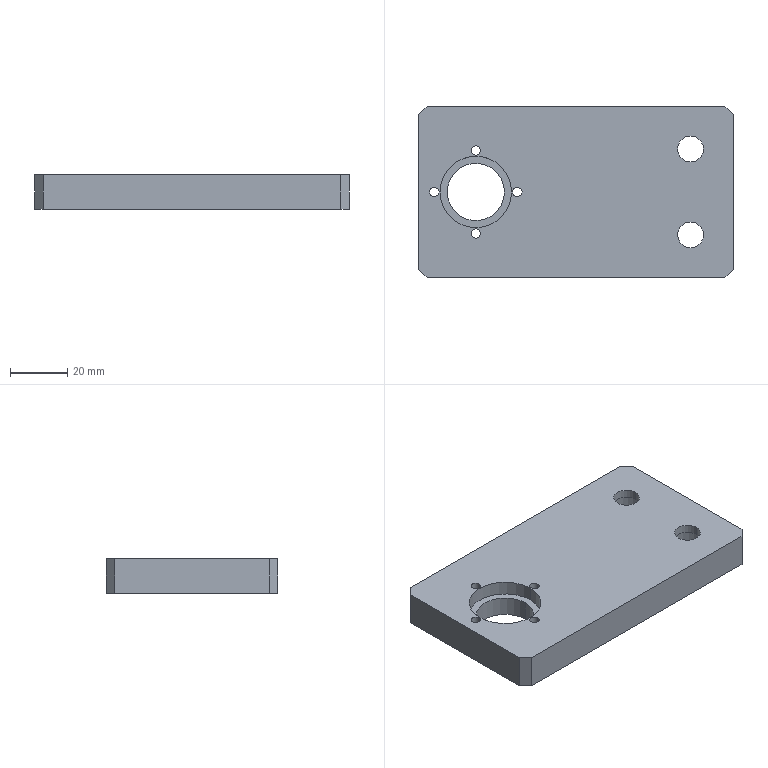Part | SolidWorks | features Cut 2, HoleWzd 2, Chamfer 1, Extrusion 1 | 1 solid | 33 faces | box 110 x 60 x 12 mm | volume 70357 mm3 | cylinder 20 | plane 13 | commonest cylinder face diameters 3.3 x8 9 x4 15 x4 20 x2 25 x2
STEP:
#1=CARTESIAN_POINT('',(47.5,15.,9.));
#2=VERTEX_POINT('',#1);
#3=CARTESIAN_POINT('',(32.5,15.,9.));
#4=VERTEX_POINT('',#3);
#5=CARTESIAN_POINT('',(40.,15.,9.));
#6=DIRECTION('',(0.,0.,-1.));
#7=DIRECTION('',(-1.,0.,0.));
#8=AXIS2_PLACEMENT_3D('',#5,#6,#7);
#9=CIRCLE('',#8,7.5);
#10=EDGE_CURVE('',#2,#4,#9,.T.);
#11=ORIENTED_EDGE('',*,*,#10,.F.);
#12=CARTESIAN_POINT('',(47.5,15.,0.));
#13=VERTEX_POINT('',#12);
#14=CARTESIAN_POINT('',(47.5,15.,0.));
#15=DIRECTION('',(0.,0.,-1.));
#16=VECTOR('',#15,1000.);
#17=LINE('',#14,#16);
#18=EDGE_CURVE('',#2,#13,#17,.T.);
#19=ORIENTED_EDGE('',*,*,#18,.T.);
#20=CARTESIAN_POINT('',(32.5,15.,0.));
#21=VERTEX_POINT('',#20);
#22=CARTESIAN_POINT('',(40.,15.,0.));
#23=DIRECTION('',(0.,0.,-1.));
#24=DIRECTION('',(-1.,0.,0.));
#25=AXIS2_PLACEMENT_3D('',#22,#23,#24);
#26=CIRCLE('',#25,7.5);
#27=EDGE_CURVE('',#13,#21,#26,.T.);
#28=ORIENTED_EDGE('',*,*,#27,.T.);
#29=CARTESIAN_POINT('',(32.5,15.,0.));
#30=DIRECTION('',(0.,0.,-1.));
#31=VECTOR('',#30,1000.);
#32=LINE('',#29,#31);
#33=EDGE_CURVE('',#4,#21,#32,.T.);
#34=ORIENTED_EDGE('',*,*,#33,.F.);
#35=EDGE_LOOP('',(#11,#19,#28,#34));
#36=FACE_OUTER_BOUND('',#35,.T.);
#37=CARTESIAN_POINT('',(40.,15.,0.));
#38=DIRECTION('',(0.,0.,-1.));
#39=DIRECTION('',(-1.,0.,0.));
#40=AXIS2_PLACEMENT_3D('',#37,#38,#39);
#41=CYLINDRICAL_SURFACE('',#40,7.5);
#42=ADVANCED_FACE('',(#36),#41,.F.);
#43=CARTESIAN_POINT('',(44.5,15.,12.));
#44=VERTEX_POINT('',#43);
#45=CARTESIAN_POINT('',(35.5,15.,12.));
#46=VERTEX_POINT('',#45);
#47=CARTESIAN_POINT('',(40.,15.,12.));
#48=DIRECTION('',(0.,0.,-1.));
#49=DIRECTION('',(-1.,0.,0.));
#50=AXIS2_PLACEMENT_3D('',#47,#48,#49);
#51=CIRCLE('',#50,4.5);
#52=EDGE_CURVE('',#44,#46,#51,.T.);
#53=ORIENTED_EDGE('',*,*,#52,.F.);
#54=CARTESIAN_POINT('',(44.5,15.,9.));
#55=VERTEX_POINT('',#54);
#56=CARTESIAN_POINT('',(44.5,15.,0.));
#57=DIRECTION('',(0.,0.,-1.));
#58=VECTOR('',#57,1000.);
#59=LINE('',#56,#58);
#60=EDGE_CURVE('',#44,#55,#59,.T.);
#61=ORIENTED_EDGE('',*,*,#60,.T.);
#62=CARTESIAN_POINT('',(35.5,15.,9.));
#63=VERTEX_POINT('',#62);
#64=CARTESIAN_POINT('',(40.,15.,9.));
#65=DIRECTION('',(0.,0.,-1.));
#66=DIRECTION('',(-1.,0.,0.));
#67=AXIS2_PLACEMENT_3D('',#64,#65,#66);
#68=CIRCLE('',#67,4.5);
#69=EDGE_CURVE('',#55,#63,#68,.T.);
#70=ORIENTED_EDGE('',*,*,#69,.T.);
#71=CARTESIAN_POINT('',(35.5,15.,0.));
#72=DIRECTION('',(0.,0.,-1.));
#73=VECTOR('',#72,1000.);
#74=LINE('',#71,#73);
#75=EDGE_CURVE('',#46,#63,#74,.T.);
#76=ORIENTED_EDGE('',*,*,#75,.F.);
#77=EDGE_LOOP('',(#53,#61,#70,#76));
#78=FACE_OUTER_BOUND('',#77,.T.);
#79=CARTESIAN_POINT('',(40.,15.,0.));
#80=DIRECTION('',(0.,0.,-1.));
#81=DIRECTION('',(-1.,0.,0.));
#82=AXIS2_PLACEMENT_3D('',#79,#80,#81);
#83=CYLINDRICAL_SURFACE('',#82,4.5);
#84=ADVANCED_FACE('',(#78),#83,.F.);
#85=CARTESIAN_POINT('',(47.5,-15.,9.));
#86=VERTEX_POINT('',#85);
#87=CARTESIAN_POINT('',(32.5,-15.,9.));
#88=VERTEX_POINT('',#87);
#89=CARTESIAN_POINT('',(40.,-15.,9.));
#90=DIRECTION('',(0.,0.,-1.));
#91=DIRECTION('',(-1.,0.,0.));
#92=AXIS2_PLACEMENT_3D('',#89,#90,#91);
#93=CIRCLE('',#92,7.5);
#94=EDGE_CURVE('',#86,#88,#93,.T.);
#95=ORIENTED_EDGE('',*,*,#94,.F.);
#96=CARTESIAN_POINT('',(47.5,-15.,0.));
#97=VERTEX_POINT('',#96);
#98=CARTESIAN_POINT('',(47.5,-15.,0.));
#99=DIRECTION('',(0.,0.,-1.));
#100=VECTOR('',#99,1000.);
#101=LINE('',#98,#100);
#102=EDGE_CURVE('',#86,#97,#101,.T.);
#103=ORIENTED_EDGE('',*,*,#102,.T.);
#104=CARTESIAN_POINT('',(32.5,-15.,0.));
#105=VERTEX_POINT('',#104);
#106=CARTESIAN_POINT('',(40.,-15.,0.));
#107=DIRECTION('',(0.,0.,-1.));
#108=DIRECTION('',(-1.,0.,0.));
#109=AXIS2_PLACEMENT_3D('',#106,#107,#108);
#110=CIRCLE('',#109,7.5);
#111=EDGE_CURVE('',#97,#105,#110,.T.);
#112=ORIENTED_EDGE('',*,*,#111,.T.);
#113=CARTESIAN_POINT('',(32.5,-15.,0.));
#114=DIRECTION('',(0.,0.,-1.));
#115=VECTOR('',#114,1000.);
#116=LINE('',#113,#115);
#117=EDGE_CURVE('',#88,#105,#116,.T.);
#118=ORIENTED_EDGE('',*,*,#117,.F.);
#119=EDGE_LOOP('',(#95,#103,#112,#118));
#120=FACE_OUTER_BOUND('',#119,.T.);
#121=CARTESIAN_POINT('',(40.,-15.,0.));
#122=DIRECTION('',(0.,0.,-1.));
#123=DIRECTION('',(-1.,0.,0.));
#124=AXIS2_PLACEMENT_3D('',#121,#122,#123);
#125=CYLINDRICAL_SURFACE('',#124,7.5);
#126=ADVANCED_FACE('',(#120),#125,.F.);
#127=CARTESIAN_POINT('',(44.5,-15.,12.));
#128=VERTEX_POINT('',#127);
#129=CARTESIAN_POINT('',(35.5,-15.,12.));
#130=VERTEX_POINT('',#129);
#131=CARTESIAN_POINT('',(40.,-15.,12.));
#132=DIRECTION('',(0.,0.,-1.));
#133=DIRECTION('',(-1.,0.,0.));
#134=AXIS2_PLACEMENT_3D('',#131,#132,#133);
#135=CIRCLE('',#134,4.5);
#136=EDGE_CURVE('',#128,#130,#135,.T.);
#137=ORIENTED_EDGE('',*,*,#136,.F.);
#138=CARTESIAN_POINT('',(44.5,-15.,9.));
#139=VERTEX_POINT('',#138);
#140=CARTESIAN_POINT('',(44.5,-15.,0.));
#141=DIRECTION('',(0.,0.,-1.));
#142=VECTOR('',#141,1000.);
#143=LINE('',#140,#142);
#144=EDGE_CURVE('',#128,#139,#143,.T.);
#145=ORIENTED_EDGE('',*,*,#144,.T.);
#146=CARTESIAN_POINT('',(35.5,-15.,9.));
#147=VERTEX_POINT('',#146);
#148=CARTESIAN_POINT('',(40.,-15.,9.));
#149=DIRECTION('',(0.,0.,-1.));
#150=DIRECTION('',(-1.,0.,0.));
#151=AXIS2_PLACEMENT_3D('',#148,#149,#150);
#152=CIRCLE('',#151,4.5);
#153=EDGE_CURVE('',#139,#147,#152,.T.);
#154=ORIENTED_EDGE('',*,*,#153,.T.);
#155=CARTESIAN_POINT('',(35.5,-15.,0.));
#156=DIRECTION('',(0.,0.,-1.));
#157=VECTOR('',#156,1000.);
#158=LINE('',#155,#157);
#159=EDGE_CURVE('',#130,#147,#158,.T.);
#160=ORIENTED_EDGE('',*,*,#159,.F.);
#161=EDGE_LOOP('',(#137,#145,#154,#160));
#162=FACE_OUTER_BOUND('',#161,.T.);
#163=CARTESIAN_POINT('',(40.,-15.,0.));
#164=DIRECTION('',(0.,0.,-1.));
#165=DIRECTION('',(-1.,0.,0.));
#166=AXIS2_PLACEMENT_3D('',#163,#164,#165);
#167=CYLINDRICAL_SURFACE('',#166,4.5);
#168=ADVANCED_FACE('',(#162),#167,.F.);
#169=CARTESIAN_POINT('',(-36.65,14.5,0.));
#170=VERTEX_POINT('',#169);
#171=CARTESIAN_POINT('',(-33.35,14.5,0.));
#172=VERTEX_POINT('',#171);
#173=CARTESIAN_POINT('',(-35.,14.5,0.));
#174=DIRECTION('',(0.,0.,1.));
#175=DIRECTION('',(1.,0.,0.));
#176=AXIS2_PLACEMENT_3D('',#173,#174,#175);
#177=CIRCLE('',#176,1.65);
#178=EDGE_CURVE('',#170,#172,#177,.T.);
#179=ORIENTED_EDGE('',*,*,#178,.F.);
#180=CARTESIAN_POINT('',(-36.65,14.5,12.));
#181=VERTEX_POINT('',#180);
#182=CARTESIAN_POINT('',(-36.65,14.5,12.));
#183=DIRECTION('',(0.,0.,1.));
#184=VECTOR('',#183,1000.);
#185=LINE('',#182,#184);
#186=EDGE_CURVE('',#170,#181,#185,.T.);
#187=ORIENTED_EDGE('',*,*,#186,.T.);
#188=CARTESIAN_POINT('',(-33.35,14.5,12.));
#189=VERTEX_POINT('',#188);
#190=CARTESIAN_POINT('',(-35.,14.5,12.));
#191=DIRECTION('',(0.,0.,1.));
#192=DIRECTION('',(1.,0.,0.));
#193=AXIS2_PLACEMENT_3D('',#190,#191,#192);
#194=CIRCLE('',#193,1.65);
#195=EDGE_CURVE('',#181,#189,#194,.T.);
#196=ORIENTED_EDGE('',*,*,#195,.T.);
#197=CARTESIAN_POINT('',(-33.35,14.5,12.));
#198=DIRECTION('',(0.,0.,1.));
#199=VECTOR('',#198,1000.);
#200=LINE('',#197,#199);
#201=EDGE_CURVE('',#172,#189,#200,.T.);
#202=ORIENTED_EDGE('',*,*,#201,.F.);
#203=EDGE_LOOP('',(#179,#187,#196,#202));
#204=FACE_OUTER_BOUND('',#203,.T.);
#205=CARTESIAN_POINT('',(-35.,14.5,12.));
#206=DIRECTION('',(0.,0.,1.));
#207=DIRECTION('',(1.,0.,0.));
#208=AXIS2_PLACEMENT_3D('',#205,#206,#207);
#209=CYLINDRICAL_SURFACE('',#208,1.65);
#210=ADVANCED_FACE('',(#204),#209,.F.);
#211=CARTESIAN_POINT('',(-22.15,0.,0.));
#212=VERTEX_POINT('',#211);
#213=CARTESIAN_POINT('',(-18.85,0.,0.));
#214=VERTEX_POINT('',#213);
#215=CARTESIAN_POINT('',(-20.5,0.,0.));
#216=DIRECTION('',(0.,0.,1.));
#217=DIRECTION('',(1.,0.,0.));
#218=AXIS2_PLACEMENT_3D('',#215,#216,#217);
#219=CIRCLE('',#218,1.65);
#220=EDGE_CURVE('',#212,#214,#219,.T.);
#221=ORIENTED_EDGE('',*,*,#220,.F.);
#222=CARTESIAN_POINT('',(-22.15,0.,12.));
#223=VERTEX_POINT('',#222);
#224=CARTESIAN_POINT('',(-22.15,0.,12.));
#225=DIRECTION('',(0.,0.,1.));
#226=VECTOR('',#225,1000.);
#227=LINE('',#224,#226);
#228=EDGE_CURVE('',#212,#223,#227,.T.);
#229=ORIENTED_EDGE('',*,*,#228,.T.);
#230=CARTESIAN_POINT('',(-18.85,0.,12.));
#231=VERTEX_POINT('',#230);
#232=CARTESIAN_POINT('',(-20.5,0.,12.));
#233=DIRECTION('',(0.,0.,1.));
#234=DIRECTION('',(1.,0.,0.));
#235=AXIS2_PLACEMENT_3D('',#232,#233,#234);
#236=CIRCLE('',#235,1.65);
#237=EDGE_CURVE('',#223,#231,#236,.T.);
#238=ORIENTED_EDGE('',*,*,#237,.T.);
#239=CARTESIAN_POINT('',(-18.85,0.,12.));
#240=DIRECTION('',(0.,0.,1.));
#241=VECTOR('',#240,1000.);
#242=LINE('',#239,#241);
#243=EDGE_CURVE('',#214,#231,#242,.T.);
#244=ORIENTED_EDGE('',*,*,#243,.F.);
#245=EDGE_LOOP('',(#221,#229,#238,#244));
#246=FACE_OUTER_BOUND('',#245,.T.);
#247=CARTESIAN_POINT('',(-20.5,0.,12.));
#248=DIRECTION('',(0.,0.,1.));
#249=DIRECTION('',(1.,0.,0.));
#250=AXIS2_PLACEMENT_3D('',#247,#248,#249);
#251=CYLINDRICAL_SURFACE('',#250,1.65);
#252=ADVANCED_FACE('',(#246),#251,.F.);
#253=CARTESIAN_POINT('',(-51.15,0.,0.));
#254=VERTEX_POINT('',#253);
#255=CARTESIAN_POINT('',(-47.85,0.,0.));
#256=VERTEX_POINT('',#255);
#257=CARTESIAN_POINT('',(-49.5,0.,0.));
#258=DIRECTION('',(0.,0.,1.));
#259=DIRECTION('',(1.,0.,0.));
#260=AXIS2_PLACEMENT_3D('',#257,#258,#259);
#261=CIRCLE('',#260,1.65);
#262=EDGE_CURVE('',#254,#256,#261,.T.);
#263=ORIENTED_EDGE('',*,*,#262,.F.);
#264=CARTESIAN_POINT('',(-51.15,0.,12.));
#265=VERTEX_POINT('',#264);
#266=CARTESIAN_POINT('',(-51.15,0.,12.));
#267=DIRECTION('',(0.,0.,1.));
#268=VECTOR('',#267,1000.);
#269=LINE('',#266,#268);
#270=EDGE_CURVE('',#254,#265,#269,.T.);
#271=ORIENTED_EDGE('',*,*,#270,.T.);
#272=CARTESIAN_POINT('',(-47.85,0.,12.));
#273=VERTEX_POINT('',#272);
#274=CARTESIAN_POINT('',(-49.5,0.,12.));
#275=DIRECTION('',(0.,0.,1.));
#276=DIRECTION('',(1.,0.,0.));
#277=AXIS2_PLACEMENT_3D('',#274,#275,#276);
#278=CIRCLE('',#277,1.65);
#279=EDGE_CURVE('',#265,#273,#278,.T.);
#280=ORIENTED_EDGE('',*,*,#279,.T.);
#281=CARTESIAN_POINT('',(-47.85,0.,12.));
#282=DIRECTION('',(0.,0.,1.));
#283=VECTOR('',#282,1000.);
#284=LINE('',#281,#283);
#285=EDGE_CURVE('',#256,#273,#284,.T.);
#286=ORIENTED_EDGE('',*,*,#285,.F.);
#287=EDGE_LOOP('',(#263,#271,#280,#286));
#288=FACE_OUTER_BOUND('',#287,.T.);
#289=CARTESIAN_POINT('',(-49.5,0.,12.));
#290=DIRECTION('',(0.,0.,1.));
#291=DIRECTION('',(1.,0.,0.));
#292=AXIS2_PLACEMENT_3D('',#289,#290,#291);
#293=CYLINDRICAL_SURFACE('',#292,1.65);
#294=ADVANCED_FACE('',(#288),#293,.F.);
#295=CARTESIAN_POINT('',(-36.65,-14.5,0.));
#296=VERTEX_POINT('',#295);
#297=CARTESIAN_POINT('',(-33.35,-14.5,0.));
#298=VERTEX_POINT('',#297);
#299=CARTESIAN_POINT('',(-35.,-14.5,0.));
#300=DIRECTION('',(0.,0.,1.));
#301=DIRECTION('',(1.,0.,0.));
#302=AXIS2_PLACEMENT_3D('',#299,#300,#301);
#303=CIRCLE('',#302,1.65);
#304=EDGE_CURVE('',#296,#298,#303,.T.);
#305=ORIENTED_EDGE('',*,*,#304,.F.);
#306=CARTESIAN_POINT('',(-36.65,-14.5,12.));
#307=VERTEX_POINT('',#306);
#308=CARTESIAN_POINT('',(-36.65,-14.5,12.));
#309=DIRECTION('',(0.,0.,1.));
#310=VECTOR('',#309,1000.);
#311=LINE('',#308,#310);
#312=EDGE_CURVE('',#296,#307,#311,.T.);
#313=ORIENTED_EDGE('',*,*,#312,.T.);
#314=CARTESIAN_POINT('',(-33.35,-14.5,12.));
#315=VERTEX_POINT('',#314);
#316=CARTESIAN_POINT('',(-35.,-14.5,12.));
#317=DIRECTION('',(0.,0.,1.));
#318=DIRECTION('',(1.,0.,0.));
#319=AXIS2_PLACEMENT_3D('',#316,#317,#318);
#320=CIRCLE('',#319,1.65);
#321=EDGE_CURVE('',#307,#315,#320,.T.);
#322=ORIENTED_EDGE('',*,*,#321,.T.);
#323=CARTESIAN_POINT('',(-33.35,-14.5,12.));
#324=DIRECTION('',(0.,0.,1.));
#325=VECTOR('',#324,1000.);
#326=LINE('',#323,#325);
#327=EDGE_CURVE('',#298,#315,#326,.T.);
#328=ORIENTED_EDGE('',*,*,#327,.F.);
#329=EDGE_LOOP('',(#305,#313,#322,#328));
#330=FACE_OUTER_BOUND('',#329,.T.);
#331=CARTESIAN_POINT('',(-35.,-14.5,12.));
#332=DIRECTION('',(0.,0.,1.));
#333=DIRECTION('',(1.,0.,0.));
#334=AXIS2_PLACEMENT_3D('',#331,#332,#333);
#335=CYLINDRICAL_SURFACE('',#334,1.65);
#336=ADVANCED_FACE('',(#330),#335,.F.);
#337=CARTESIAN_POINT('',(-45.,0.,0.));
#338=VERTEX_POINT('',#337);
#339=CARTESIAN_POINT('',(-25.,0.,0.));
#340=VERTEX_POINT('',#339);
#341=CARTESIAN_POINT('',(-35.,0.,0.));
#342=DIRECTION('',(0.,0.,1.));
#343=DIRECTION('',(1.,0.,0.));
#344=AXIS2_PLACEMENT_3D('',#341,#342,#343);
#345=CIRCLE('',#344,10.);
#346=EDGE_CURVE('',#338,#340,#345,.T.);
#347=ORIENTED_EDGE('',*,*,#346,.F.);
#348=CARTESIAN_POINT('',(-45.,0.,7.));
#349=VERTEX_POINT('',#348);
#350=CARTESIAN_POINT('',(-45.,0.,0.));
#351=DIRECTION('',(0.,0.,1.));
#352=VECTOR('',#351,1000.);
#353=LINE('',#350,#352);
#354=EDGE_CURVE('',#338,#349,#353,.T.);
#355=ORIENTED_EDGE('',*,*,#354,.T.);
#356=CARTESIAN_POINT('',(-25.,0.,7.));
#357=VERTEX_POINT('',#356);
#358=CARTESIAN_POINT('',(-35.,0.,7.));
#359=DIRECTION('',(0.,0.,-1.));
#360=DIRECTION('',(-1.,0.,0.));
#361=AXIS2_PLACEMENT_3D('',#358,#359,#360);
#362=CIRCLE('',#361,10.);
#363=EDGE_CURVE('',#357,#349,#362,.T.);
#364=ORIENTED_EDGE('',*,*,#363,.F.);
#365=CARTESIAN_POINT('',(-25.,0.,0.));
#366=DIRECTION('',(0.,0.,1.));
#367=VECTOR('',#366,1000.);
#368=LINE('',#365,#367);
#369=EDGE_CURVE('',#340,#357,#368,.T.);
#370=ORIENTED_EDGE('',*,*,#369,.F.);
#371=EDGE_LOOP('',(#347,#355,#364,#370));
#372=FACE_OUTER_BOUND('',#371,.T.);
#373=CARTESIAN_POINT('',(-35.,0.,0.));
#374=DIRECTION('',(0.,0.,1.));
#375=DIRECTION('',(1.,0.,0.));
#376=AXIS2_PLACEMENT_3D('',#373,#374,#375);
#377=CYLINDRICAL_SURFACE('',#376,10.);
#378=ADVANCED_FACE('',(#372),#377,.F.);
#379=CARTESIAN_POINT('',(-22.5,0.,7.));
#380=VERTEX_POINT('',#379);
#381=CARTESIAN_POINT('',(-47.5,0.,7.));
#382=VERTEX_POINT('',#381);
#383=CARTESIAN_POINT('',(-35.,0.,7.));
#384=DIRECTION('',(0.,0.,-1.));
#385=DIRECTION('',(-1.,0.,0.));
#386=AXIS2_PLACEMENT_3D('',#383,#384,#385);
#387=CIRCLE('',#386,12.5);
#388=EDGE_CURVE('',#380,#382,#387,.T.);
#389=ORIENTED_EDGE('',*,*,#388,.T.);
#390=CARTESIAN_POINT('',(-47.5,0.,12.));
#391=VERTEX_POINT('',#390);
#392=CARTESIAN_POINT('',(-47.5,0.,7.));
#393=DIRECTION('',(0.,0.,1.));
#394=VECTOR('',#393,1000.);
#395=LINE('',#392,#394);
#396=EDGE_CURVE('',#382,#391,#395,.T.);
#397=ORIENTED_EDGE('',*,*,#396,.T.);
#398=CARTESIAN_POINT('',(-22.5,0.,12.));
#399=VERTEX_POINT('',#398);
#400=CARTESIAN_POINT('',(-35.,0.,12.));
#401=DIRECTION('',(0.,0.,-1.));
#402=DIRECTION('',(-1.,0.,0.));
#403=AXIS2_PLACEMENT_3D('',#400,#401,#402);
#404=CIRCLE('',#403,12.5);
#405=EDGE_CURVE('',#399,#391,#404,.T.);
#406=ORIENTED_EDGE('',*,*,#405,.F.);
#407=CARTESIAN_POINT('',(-22.5,0.,7.));
#408=DIRECTION('',(0.,0.,1.));
#409=VECTOR('',#408,1000.);
#410=LINE('',#407,#409);
#411=EDGE_CURVE('',#380,#399,#410,.T.);
#412=ORIENTED_EDGE('',*,*,#411,.F.);
#413=EDGE_LOOP('',(#389,#397,#406,#412));
#414=FACE_OUTER_BOUND('',#413,.T.);
#415=CARTESIAN_POINT('',(-35.,0.,7.));
#416=DIRECTION('',(0.,0.,1.));
#417=DIRECTION('',(1.,0.,0.));
#418=AXIS2_PLACEMENT_3D('',#415,#416,#417);
#419=CYLINDRICAL_SURFACE('',#418,12.5);
#420=ADVANCED_FACE('',(#414),#419,.F.);
#421=CARTESIAN_POINT('',(55.,-27.,0.));
#422=VERTEX_POINT('',#421);
#423=CARTESIAN_POINT('',(55.,27.,0.));
#424=VERTEX_POINT('',#423);
#425=CARTESIAN_POINT('',(55.,-30.,0.));
#426=DIRECTION('',(0.,1.,0.));
#427=VECTOR('',#426,1000.);
#428=LINE('',#425,#427);
#429=EDGE_CURVE('',#422,#424,#428,.T.);
#430=ORIENTED_EDGE('',*,*,#429,.T.);
#431=CARTESIAN_POINT('',(55.,27.,12.));
#432=VERTEX_POINT('',#431);
#433=CARTESIAN_POINT('',(55.,27.,12.));
#434=DIRECTION('',(0.,0.,1.));
#435=VECTOR('',#434,1000.);
#436=LINE('',#433,#435);
#437=EDGE_CURVE('',#424,#432,#436,.T.);
#438=ORIENTED_EDGE('',*,*,#437,.T.);
#439=CARTESIAN_POINT('',(55.,-27.,12.));
#440=VERTEX_POINT('',#439);
#441=CARTESIAN_POINT('',(55.,-30.,12.));
#442=DIRECTION('',(0.,1.,0.));
#443=VECTOR('',#442,1000.);
#444=LINE('',#441,#443);
#445=EDGE_CURVE('',#440,#432,#444,.T.);
#446=ORIENTED_EDGE('',*,*,#445,.F.);
#447=CARTESIAN_POINT('',(55.,-27.,12.));
#448=DIRECTION('',(0.,0.,-1.));
#449=VECTOR('',#448,1000.);
#450=LINE('',#447,#449);
#451=EDGE_CURVE('',#440,#422,#450,.T.);
#452=ORIENTED_EDGE('',*,*,#451,.T.);
#453=EDGE_LOOP('',(#430,#438,#446,#452));
#454=FACE_OUTER_BOUND('',#453,.T.);
#455=CARTESIAN_POINT('',(55.,-30.,12.));
#456=DIRECTION('',(-1.,0.,0.));
#457=DIRECTION('',(0.,0.,1.));
#458=AXIS2_PLACEMENT_3D('',#455,#456,#457);
#459=PLANE('',#458);
#460=ADVANCED_FACE('',(#454),#459,.F.);
#461=CARTESIAN_POINT('',(52.,30.,0.));
#462=VERTEX_POINT('',#461);
#463=CARTESIAN_POINT('',(-52.,30.,0.));
#464=VERTEX_POINT('',#463);
#465=CARTESIAN_POINT('',(-55.,30.,0.));
#466=DIRECTION('',(-1.,0.,0.));
#467=VECTOR('',#466,1000.);
#468=LINE('',#465,#467);
#469=EDGE_CURVE('',#462,#464,#468,.T.);
#470=ORIENTED_EDGE('',*,*,#469,.T.);
#471=CARTESIAN_POINT('',(-52.,30.,12.));
#472=VERTEX_POINT('',#471);
#473=CARTESIAN_POINT('',(-52.,30.,12.));
#474=DIRECTION('',(0.,0.,1.));
#475=VECTOR('',#474,1000.);
#476=LINE('',#473,#475);
#477=EDGE_CURVE('',#464,#472,#476,.T.);
#478=ORIENTED_EDGE('',*,*,#477,.T.);
#479=CARTESIAN_POINT('',(52.,30.,12.));
#480=VERTEX_POINT('',#479);
#481=CARTESIAN_POINT('',(-55.,30.,12.));
#482=DIRECTION('',(-1.,0.,0.));
#483=VECTOR('',#482,1000.);
#484=LINE('',#481,#483);
#485=EDGE_CURVE('',#480,#472,#484,.T.);
#486=ORIENTED_EDGE('',*,*,#485,.F.);
#487=CARTESIAN_POINT('',(52.,30.,12.));
#488=DIRECTION('',(0.,0.,-1.));
#489=VECTOR('',#488,1000.);
#490=LINE('',#487,#489);
#491=EDGE_CURVE('',#480,#462,#490,.T.);
#492=ORIENTED_EDGE('',*,*,#491,.T.);
#493=EDGE_LOOP('',(#470,#478,#486,#492));
#494=FACE_OUTER_BOUND('',#493,.T.);
#495=CARTESIAN_POINT('',(-55.,30.,12.));
#496=DIRECTION('',(0.,-1.,0.));
#497=DIRECTION('',(0.,0.,-1.));
#498=AXIS2_PLACEMENT_3D('',#495,#496,#497);
#499=PLANE('',#498);
#500=ADVANCED_FACE('',(#494),#499,.F.);
#501=CARTESIAN_POINT('',(-55.,27.,0.));
#502=VERTEX_POINT('',#501);
#503=CARTESIAN_POINT('',(-55.,-27.,0.));
#504=VERTEX_POINT('',#503);
#505=CARTESIAN_POINT('',(-55.,-30.,0.));
#506=DIRECTION('',(0.,-1.,0.));
#507=VECTOR('',#506,1000.);
#508=LINE('',#505,#507);
#509=EDGE_CURVE('',#502,#504,#508,.T.);
#510=ORIENTED_EDGE('',*,*,#509,.T.);
#511=CARTESIAN_POINT('',(-55.,-27.,12.));
#512=VERTEX_POINT('',#511);
#513=CARTESIAN_POINT('',(-55.,-27.,12.));
#514=DIRECTION('',(0.,0.,1.));
#515=VECTOR('',#514,1000.);
#516=LINE('',#513,#515);
#517=EDGE_CURVE('',#504,#512,#516,.T.);
#518=ORIENTED_EDGE('',*,*,#517,.T.);
#519=CARTESIAN_POINT('',(-55.,27.,12.));
#520=VERTEX_POINT('',#519);
#521=CARTESIAN_POINT('',(-55.,-30.,12.));
#522=DIRECTION('',(0.,-1.,0.));
#523=VECTOR('',#522,1000.);
#524=LINE('',#521,#523);
#525=EDGE_CURVE('',#520,#512,#524,.T.);
#526=ORIENTED_EDGE('',*,*,#525,.F.);
#527=CARTESIAN_POINT('',(-55.,27.,12.));
#528=DIRECTION('',(0.,0.,-1.));
#529=VECTOR('',#528,1000.);
#530=LINE('',#527,#529);
#531=EDGE_CURVE('',#520,#502,#530,.T.);
#532=ORIENTED_EDGE('',*,*,#531,.T.);
#533=EDGE_LOOP('',(#510,#518,#526,#532));
#534=FACE_OUTER_BOUND('',#533,.T.);
#535=CARTESIAN_POINT('',(-55.,-30.,12.));
#536=DIRECTION('',(1.,0.,0.));
#537=DIRECTION('',(0.,0.,-1.));
#538=AXIS2_PLACEMENT_3D('',#535,#536,#537);
#539=PLANE('',#538);
#540=ADVANCED_FACE('',(#534),#539,.F.);
#541=CARTESIAN_POINT('',(-52.,-30.,12.));
#542=VERTEX_POINT('',#541);
#543=CARTESIAN_POINT('',(52.,-30.,12.));
#544=VERTEX_POINT('',#543);
#545=CARTESIAN_POINT('',(-55.,-30.,12.));
#546=DIRECTION('',(1.,0.,0.));
#547=VECTOR('',#546,1000.);
#548=LINE('',#545,#547);
#549=EDGE_CURVE('',#542,#544,#548,.T.);
#550=ORIENTED_EDGE('',*,*,#549,.F.);
#551=CARTESIAN_POINT('',(-52.,-30.,0.));
#552=VERTEX_POINT('',#551);
#553=CARTESIAN_POINT('',(-52.,-30.,12.));
#554=DIRECTION('',(0.,0.,-1.));
#555=VECTOR('',#554,1000.);
#556=LINE('',#553,#555);
#557=EDGE_CURVE('',#542,#552,#556,.T.);
#558=ORIENTED_EDGE('',*,*,#557,.T.);
#559=CARTESIAN_POINT('',(52.,-30.,0.));
#560=VERTEX_POINT('',#559);
#561=CARTESIAN_POINT('',(-55.,-30.,0.));
#562=DIRECTION('',(1.,0.,0.));
#563=VECTOR('',#562,1000.);
#564=LINE('',#561,#563);
#565=EDGE_CURVE('',#552,#560,#564,.T.);
#566=ORIENTED_EDGE('',*,*,#565,.T.);
#567=CARTESIAN_POINT('',(52.,-30.,12.));
#568=DIRECTION('',(0.,0.,1.));
#569=VECTOR('',#568,1000.);
#570=LINE('',#567,#569);
#571=EDGE_CURVE('',#560,#544,#570,.T.);
#572=ORIENTED_EDGE('',*,*,#571,.T.);
#573=EDGE_LOOP('',(#550,#558,#566,#572));
#574=FACE_OUTER_BOUND('',#573,.T.);
#575=CARTESIAN_POINT('',(-55.,-30.,12.));
#576=DIRECTION('',(0.,1.,0.));
#577=DIRECTION('',(0.,0.,1.));
#578=AXIS2_PLACEMENT_3D('',#575,#576,#577);
#579=PLANE('',#578);
#580=ADVANCED_FACE('',(#574),#579,.F.);
#581=CARTESIAN_POINT('',(40.,15.,12.));
#582=DIRECTION('',(0.,0.,-1.));
#583=DIRECTION('',(-1.,0.,0.));
#584=AXIS2_PLACEMENT_3D('',#581,#582,#583);
#585=CIRCLE('',#584,4.5);
#586=EDGE_CURVE('',#46,#44,#585,.T.);
#587=ORIENTED_EDGE('',*,*,#586,.T.);
#588=ORIENTED_EDGE('',*,*,#52,.T.);
#589=EDGE_LOOP('',(#587,#588));
#590=FACE_BOUND('',#589,.T.);
#591=CARTESIAN_POINT('',(40.,-15.,12.));
#592=DIRECTION('',(0.,0.,-1.));
#593=DIRECTION('',(-1.,0.,0.));
#594=AXIS2_PLACEMENT_3D('',#591,#592,#593);
#595=CIRCLE('',#594,4.5);
#596=EDGE_CURVE('',#130,#128,#595,.T.);
#597=ORIENTED_EDGE('',*,*,#596,.T.);
#598=ORIENTED_EDGE('',*,*,#136,.T.);
#599=EDGE_LOOP('',(#597,#598));
#600=FACE_BOUND('',#599,.T.);
#601=CARTESIAN_POINT('',(-35.,14.5,12.));
#602=DIRECTION('',(0.,0.,1.));
#603=DIRECTION('',(1.,0.,0.));
#604=AXIS2_PLACEMENT_3D('',#601,#602,#603);
#605=CIRCLE('',#604,1.65);
#606=EDGE_CURVE('',#189,#181,#605,.T.);
#607=ORIENTED_EDGE('',*,*,#606,.F.);
#608=ORIENTED_EDGE('',*,*,#195,.F.);
#609=EDGE_LOOP('',(#607,#608));
#610=FACE_BOUND('',#609,.T.);
#611=CARTESIAN_POINT('',(-20.5,0.,12.));
#612=DIRECTION('',(0.,0.,1.));
#613=DIRECTION('',(1.,0.,0.));
#614=AXIS2_PLACEMENT_3D('',#611,#612,#613);
#615=CIRCLE('',#614,1.65);
#616=EDGE_CURVE('',#231,#223,#615,.T.);
#617=ORIENTED_EDGE('',*,*,#616,.F.);
#618=ORIENTED_EDGE('',*,*,#237,.F.);
#619=EDGE_LOOP('',(#617,#618));
#620=FACE_BOUND('',#619,.T.);
#621=CARTESIAN_POINT('',(-49.5,0.,12.));
#622=DIRECTION('',(0.,0.,1.));
#623=DIRECTION('',(1.,0.,0.));
#624=AXIS2_PLACEMENT_3D('',#621,#622,#623);
#625=CIRCLE('',#624,1.65);
#626=EDGE_CURVE('',#273,#265,#625,.T.);
#627=ORIENTED_EDGE('',*,*,#626,.F.);
#628=ORIENTED_EDGE('',*,*,#279,.F.);
#629=EDGE_LOOP('',(#627,#628));
#630=FACE_BOUND('',#629,.T.);
#631=CARTESIAN_POINT('',(-35.,-14.5,12.));
#632=DIRECTION('',(0.,0.,1.));
#633=DIRECTION('',(1.,0.,0.));
#634=AXIS2_PLACEMENT_3D('',#631,#632,#633);
#635=CIRCLE('',#634,1.65);
#636=EDGE_CURVE('',#315,#307,#635,.T.);
#637=ORIENTED_EDGE('',*,*,#636,.F.);
#638=ORIENTED_EDGE('',*,*,#321,.F.);
#639=EDGE_LOOP('',(#637,#638));
#640=FACE_BOUND('',#639,.T.);
#641=ORIENTED_EDGE('',*,*,#405,.T.);
#642=CARTESIAN_POINT('',(-35.,0.,12.));
#643=DIRECTION('',(0.,0.,-1.));
#644=DIRECTION('',(-1.,0.,0.));
#645=AXIS2_PLACEMENT_3D('',#642,#643,#644);
#646=CIRCLE('',#645,12.5);
#647=EDGE_CURVE('',#391,#399,#646,.T.);
#648=ORIENTED_EDGE('',*,*,#647,.T.);
#649=EDGE_LOOP('',(#641,#648));
#650=FACE_BOUND('',#649,.T.);
#651=ORIENTED_EDGE('',*,*,#525,.T.);
#652=CARTESIAN_POINT('',(-52.,-30.,12.));
#653=DIRECTION('',(0.7071,-0.7071,0.));
#654=VECTOR('',#653,1000.);
#655=LINE('',#652,#654);
#656=EDGE_CURVE('',#512,#542,#655,.T.);
#657=ORIENTED_EDGE('',*,*,#656,.T.);
#658=ORIENTED_EDGE('',*,*,#549,.T.);
#659=CARTESIAN_POINT('',(55.,-27.,12.));
#660=DIRECTION('',(0.7071,0.7071,0.));
#661=VECTOR('',#660,1000.);
#662=LINE('',#659,#661);
#663=EDGE_CURVE('',#544,#440,#662,.T.);
#664=ORIENTED_EDGE('',*,*,#663,.T.);
#665=ORIENTED_EDGE('',*,*,#445,.T.);
#666=CARTESIAN_POINT('',(52.,30.,12.));
#667=DIRECTION('',(-0.7071,0.7071,0.));
#668=VECTOR('',#667,1000.);
#669=LINE('',#666,#668);
#670=EDGE_CURVE('',#432,#480,#669,.T.);
#671=ORIENTED_EDGE('',*,*,#670,.T.);
#672=ORIENTED_EDGE('',*,*,#485,.T.);
#673=CARTESIAN_POINT('',(-55.,27.,12.));
#674=DIRECTION('',(-0.7071,-0.7071,0.));
#675=VECTOR('',#674,1000.);
#676=LINE('',#673,#675);
#677=EDGE_CURVE('',#472,#520,#676,.T.);
#678=ORIENTED_EDGE('',*,*,#677,.T.);
#679=EDGE_LOOP('',(#651,#657,#658,#664,#665,#671,#672,#678));
#680=FACE_OUTER_BOUND('',#679,.T.);
#681=CARTESIAN_POINT('',(0.,0.,12.));
#682=DIRECTION('',(0.,0.,-1.));
#683=DIRECTION('',(-1.,0.,0.));
#684=AXIS2_PLACEMENT_3D('',#681,#682,#683);
#685=PLANE('',#684);
#686=ADVANCED_FACE('',(#590,#600,#610,#620,#630,#640,#650,#680),#685,.F.);
#687=CARTESIAN_POINT('',(40.,15.,0.));
#688=DIRECTION('',(0.,0.,-1.));
#689=DIRECTION('',(-1.,0.,0.));
#690=AXIS2_PLACEMENT_3D('',#687,#688,#689);
#691=CIRCLE('',#690,7.5);
#692=EDGE_CURVE('',#21,#13,#691,.T.);
#693=ORIENTED_EDGE('',*,*,#692,.F.);
#694=ORIENTED_EDGE('',*,*,#27,.F.);
#695=EDGE_LOOP('',(#693,#694));
#696=FACE_BOUND('',#695,.T.);
#697=CARTESIAN_POINT('',(40.,-15.,0.));
#698=DIRECTION('',(0.,0.,-1.));
#699=DIRECTION('',(-1.,0.,0.));
#700=AXIS2_PLACEMENT_3D('',#697,#698,#699);
#701=CIRCLE('',#700,7.5);
#702=EDGE_CURVE('',#105,#97,#701,.T.);
#703=ORIENTED_EDGE('',*,*,#702,.F.);
#704=ORIENTED_EDGE('',*,*,#111,.F.);
#705=EDGE_LOOP('',(#703,#704));
#706=FACE_BOUND('',#705,.T.);
#707=CARTESIAN_POINT('',(-35.,14.5,0.));
#708=DIRECTION('',(0.,0.,1.));
#709=DIRECTION('',(1.,0.,0.));
#710=AXIS2_PLACEMENT_3D('',#707,#708,#709);
#711=CIRCLE('',#710,1.65);
#712=EDGE_CURVE('',#172,#170,#711,.T.);
#713=ORIENTED_EDGE('',*,*,#712,.T.);
#714=ORIENTED_EDGE('',*,*,#178,.T.);
#715=EDGE_LOOP('',(#713,#714));
#716=FACE_BOUND('',#715,.T.);
#717=CARTESIAN_POINT('',(-20.5,0.,0.));
#718=DIRECTION('',(0.,0.,1.));
#719=DIRECTION('',(1.,0.,0.));
#720=AXIS2_PLACEMENT_3D('',#717,#718,#719);
#721=CIRCLE('',#720,1.65);
#722=EDGE_CURVE('',#214,#212,#721,.T.);
#723=ORIENTED_EDGE('',*,*,#722,.T.);
#724=ORIENTED_EDGE('',*,*,#220,.T.);
#725=EDGE_LOOP('',(#723,#724));
#726=FACE_BOUND('',#725,.T.);
#727=CARTESIAN_POINT('',(-49.5,0.,0.));
#728=DIRECTION('',(0.,0.,1.));
#729=DIRECTION('',(1.,0.,0.));
#730=AXIS2_PLACEMENT_3D('',#727,#728,#729);
#731=CIRCLE('',#730,1.65);
#732=EDGE_CURVE('',#256,#254,#731,.T.);
#733=ORIENTED_EDGE('',*,*,#732,.T.);
#734=ORIENTED_EDGE('',*,*,#262,.T.);
#735=EDGE_LOOP('',(#733,#734));
#736=FACE_BOUND('',#735,.T.);
#737=CARTESIAN_POINT('',(-35.,-14.5,0.));
#738=DIRECTION('',(0.,0.,1.));
#739=DIRECTION('',(1.,0.,0.));
#740=AXIS2_PLACEMENT_3D('',#737,#738,#739);
#741=CIRCLE('',#740,1.65);
#742=EDGE_CURVE('',#298,#296,#741,.T.);
#743=ORIENTED_EDGE('',*,*,#742,.T.);
#744=ORIENTED_EDGE('',*,*,#304,.T.);
#745=EDGE_LOOP('',(#743,#744));
#746=FACE_BOUND('',#745,.T.);
#747=CARTESIAN_POINT('',(-35.,0.,0.));
#748=DIRECTION('',(0.,0.,1.));
#749=DIRECTION('',(1.,0.,0.));
#750=AXIS2_PLACEMENT_3D('',#747,#748,#749);
#751=CIRCLE('',#750,10.);
#752=EDGE_CURVE('',#340,#338,#751,.T.);
#753=ORIENTED_EDGE('',*,*,#752,.T.);
#754=ORIENTED_EDGE('',*,*,#346,.T.);
#755=EDGE_LOOP('',(#753,#754));
#756=FACE_BOUND('',#755,.T.);
#757=ORIENTED_EDGE('',*,*,#565,.F.);
#758=CARTESIAN_POINT('',(-41.,-41.,0.));
#759=DIRECTION('',(-0.7071,0.7071,0.));
#760=VECTOR('',#759,1000.);
#761=LINE('',#758,#760);
#762=EDGE_CURVE('',#552,#504,#761,.T.);
#763=ORIENTED_EDGE('',*,*,#762,.T.);
#764=ORIENTED_EDGE('',*,*,#509,.F.);
#765=CARTESIAN_POINT('',(-41.,41.,0.));
#766=DIRECTION('',(0.7071,0.7071,0.));
#767=VECTOR('',#766,1000.);
#768=LINE('',#765,#767);
#769=EDGE_CURVE('',#502,#464,#768,.T.);
#770=ORIENTED_EDGE('',*,*,#769,.T.);
#771=ORIENTED_EDGE('',*,*,#469,.F.);
#772=CARTESIAN_POINT('',(41.,41.,0.));
#773=DIRECTION('',(0.7071,-0.7071,0.));
#774=VECTOR('',#773,1000.);
#775=LINE('',#772,#774);
#776=EDGE_CURVE('',#462,#424,#775,.T.);
#777=ORIENTED_EDGE('',*,*,#776,.T.);
#778=ORIENTED_EDGE('',*,*,#429,.F.);
#779=CARTESIAN_POINT('',(41.,-41.,0.));
#780=DIRECTION('',(-0.7071,-0.7071,0.));
#781=VECTOR('',#780,1000.);
#782=LINE('',#779,#781);
#783=EDGE_CURVE('',#422,#560,#782,.T.);
#784=ORIENTED_EDGE('',*,*,#783,.T.);
#785=EDGE_LOOP('',(#757,#763,#764,#770,#771,#777,#778,#784));
#786=FACE_OUTER_BOUND('',#785,.T.);
#787=CARTESIAN_POINT('',(0.,0.,0.));
#788=DIRECTION('',(0.,0.,-1.));
#789=DIRECTION('',(-1.,0.,0.));
#790=AXIS2_PLACEMENT_3D('',#787,#788,#789);
#791=PLANE('',#790);
#792=ADVANCED_FACE('',(#696,#706,#716,#726,#736,#746,#756,#786),#791,.T.);
#793=ORIENTED_EDGE('',*,*,#396,.F.);
#794=CARTESIAN_POINT('',(-35.,0.,7.));
#795=DIRECTION('',(0.,0.,-1.));
#796=DIRECTION('',(-1.,0.,0.));
#797=AXIS2_PLACEMENT_3D('',#794,#795,#796);
#798=CIRCLE('',#797,12.5);
#799=EDGE_CURVE('',#382,#380,#798,.T.);
#800=ORIENTED_EDGE('',*,*,#799,.T.);
#801=ORIENTED_EDGE('',*,*,#411,.T.);
#802=ORIENTED_EDGE('',*,*,#647,.F.);
#803=EDGE_LOOP('',(#793,#800,#801,#802));
#804=FACE_OUTER_BOUND('',#803,.T.);
#805=CARTESIAN_POINT('',(-35.,0.,7.));
#806=DIRECTION('',(0.,0.,1.));
#807=DIRECTION('',(1.,0.,0.));
#808=AXIS2_PLACEMENT_3D('',#805,#806,#807);
#809=CYLINDRICAL_SURFACE('',#808,12.5);
#810=ADVANCED_FACE('',(#804),#809,.F.);
#811=ORIENTED_EDGE('',*,*,#363,.T.);
#812=CARTESIAN_POINT('',(-35.,0.,7.));
#813=DIRECTION('',(0.,0.,-1.));
#814=DIRECTION('',(-1.,0.,0.));
#815=AXIS2_PLACEMENT_3D('',#812,#813,#814);
#816=CIRCLE('',#815,10.);
#817=EDGE_CURVE('',#349,#357,#816,.T.);
#818=ORIENTED_EDGE('',*,*,#817,.T.);
#819=EDGE_LOOP('',(#811,#818));
#820=FACE_BOUND('',#819,.T.);
#821=ORIENTED_EDGE('',*,*,#388,.F.);
#822=ORIENTED_EDGE('',*,*,#799,.F.);
#823=EDGE_LOOP('',(#821,#822));
#824=FACE_OUTER_BOUND('',#823,.T.);
#825=CARTESIAN_POINT('',(-35.,0.,7.));
#826=DIRECTION('',(0.,0.,-1.));
#827=DIRECTION('',(-1.,0.,0.));
#828=AXIS2_PLACEMENT_3D('',#825,#826,#827);
#829=PLANE('',#828);
#830=ADVANCED_FACE('',(#820,#824),#829,.F.);
#831=ORIENTED_EDGE('',*,*,#354,.F.);
#832=ORIENTED_EDGE('',*,*,#752,.F.);
#833=ORIENTED_EDGE('',*,*,#369,.T.);
#834=ORIENTED_EDGE('',*,*,#817,.F.);
#835=EDGE_LOOP('',(#831,#832,#833,#834));
#836=FACE_OUTER_BOUND('',#835,.T.);
#837=CARTESIAN_POINT('',(-35.,0.,0.));
#838=DIRECTION('',(0.,0.,1.));
#839=DIRECTION('',(1.,0.,0.));
#840=AXIS2_PLACEMENT_3D('',#837,#838,#839);
#841=CYLINDRICAL_SURFACE('',#840,10.);
#842=ADVANCED_FACE('',(#836),#841,.F.);
#843=ORIENTED_EDGE('',*,*,#656,.F.);
#844=ORIENTED_EDGE('',*,*,#517,.F.);
#845=ORIENTED_EDGE('',*,*,#762,.F.);
#846=ORIENTED_EDGE('',*,*,#557,.F.);
#847=EDGE_LOOP('',(#843,#844,#845,#846));
#848=FACE_OUTER_BOUND('',#847,.T.);
#849=CARTESIAN_POINT('',(-52.,-30.,12.));
#850=DIRECTION('',(0.7071,0.7071,0.));
#851=DIRECTION('',(0.,0.,-1.));
#852=AXIS2_PLACEMENT_3D('',#849,#850,#851);
#853=PLANE('',#852);
#854=ADVANCED_FACE('',(#848),#853,.F.);
#855=ORIENTED_EDGE('',*,*,#677,.F.);
#856=ORIENTED_EDGE('',*,*,#477,.F.);
#857=ORIENTED_EDGE('',*,*,#769,.F.);
#858=ORIENTED_EDGE('',*,*,#531,.F.);
#859=EDGE_LOOP('',(#855,#856,#857,#858));
#860=FACE_OUTER_BOUND('',#859,.T.);
#861=CARTESIAN_POINT('',(-55.,27.,12.));
#862=DIRECTION('',(0.7071,-0.7071,0.));
#863=DIRECTION('',(0.,0.,-1.));
#864=AXIS2_PLACEMENT_3D('',#861,#862,#863);
#865=PLANE('',#864);
#866=ADVANCED_FACE('',(#860),#865,.F.);
#867=ORIENTED_EDGE('',*,*,#670,.F.);
#868=ORIENTED_EDGE('',*,*,#437,.F.);
#869=ORIENTED_EDGE('',*,*,#776,.F.);
#870=ORIENTED_EDGE('',*,*,#491,.F.);
#871=EDGE_LOOP('',(#867,#868,#869,#870));
#872=FACE_OUTER_BOUND('',#871,.T.);
#873=CARTESIAN_POINT('',(52.,30.,12.));
#874=DIRECTION('',(-0.7071,-0.7071,0.));
#875=DIRECTION('',(0.,0.,-1.));
#876=AXIS2_PLACEMENT_3D('',#873,#874,#875);
#877=PLANE('',#876);
#878=ADVANCED_FACE('',(#872),#877,.F.);
#879=ORIENTED_EDGE('',*,*,#663,.F.);
#880=ORIENTED_EDGE('',*,*,#571,.F.);
#881=ORIENTED_EDGE('',*,*,#783,.F.);
#882=ORIENTED_EDGE('',*,*,#451,.F.);
#883=EDGE_LOOP('',(#879,#880,#881,#882));
#884=FACE_OUTER_BOUND('',#883,.T.);
#885=CARTESIAN_POINT('',(55.,-27.,12.));
#886=DIRECTION('',(-0.7071,0.7071,0.));
#887=DIRECTION('',(0.,0.,-1.));
#888=AXIS2_PLACEMENT_3D('',#885,#886,#887);
#889=PLANE('',#888);
#890=ADVANCED_FACE('',(#884),#889,.F.);
#891=ORIENTED_EDGE('',*,*,#312,.F.);
#892=ORIENTED_EDGE('',*,*,#742,.F.);
#893=ORIENTED_EDGE('',*,*,#327,.T.);
#894=ORIENTED_EDGE('',*,*,#636,.T.);
#895=EDGE_LOOP('',(#891,#892,#893,#894));
#896=FACE_OUTER_BOUND('',#895,.T.);
#897=CARTESIAN_POINT('',(-35.,-14.5,12.));
#898=DIRECTION('',(0.,0.,1.));
#899=DIRECTION('',(1.,0.,0.));
#900=AXIS2_PLACEMENT_3D('',#897,#898,#899);
#901=CYLINDRICAL_SURFACE('',#900,1.65);
#902=ADVANCED_FACE('',(#896),#901,.F.);
#903=ORIENTED_EDGE('',*,*,#270,.F.);
#904=ORIENTED_EDGE('',*,*,#732,.F.);
#905=ORIENTED_EDGE('',*,*,#285,.T.);
#906=ORIENTED_EDGE('',*,*,#626,.T.);
#907=EDGE_LOOP('',(#903,#904,#905,#906));
#908=FACE_OUTER_BOUND('',#907,.T.);
#909=CARTESIAN_POINT('',(-49.5,0.,12.));
#910=DIRECTION('',(0.,0.,1.));
#911=DIRECTION('',(1.,0.,0.));
#912=AXIS2_PLACEMENT_3D('',#909,#910,#911);
#913=CYLINDRICAL_SURFACE('',#912,1.65);
#914=ADVANCED_FACE('',(#908),#913,.F.);
#915=ORIENTED_EDGE('',*,*,#228,.F.);
#916=ORIENTED_EDGE('',*,*,#722,.F.);
#917=ORIENTED_EDGE('',*,*,#243,.T.);
#918=ORIENTED_EDGE('',*,*,#616,.T.);
#919=EDGE_LOOP('',(#915,#916,#917,#918));
#920=FACE_OUTER_BOUND('',#919,.T.);
#921=CARTESIAN_POINT('',(-20.5,0.,12.));
#922=DIRECTION('',(0.,0.,1.));
#923=DIRECTION('',(1.,0.,0.));
#924=AXIS2_PLACEMENT_3D('',#921,#922,#923);
#925=CYLINDRICAL_SURFACE('',#924,1.65);
#926=ADVANCED_FACE('',(#920),#925,.F.);
#927=ORIENTED_EDGE('',*,*,#186,.F.);
#928=ORIENTED_EDGE('',*,*,#712,.F.);
#929=ORIENTED_EDGE('',*,*,#201,.T.);
#930=ORIENTED_EDGE('',*,*,#606,.T.);
#931=EDGE_LOOP('',(#927,#928,#929,#930));
#932=FACE_OUTER_BOUND('',#931,.T.);
#933=CARTESIAN_POINT('',(-35.,14.5,12.));
#934=DIRECTION('',(0.,0.,1.));
#935=DIRECTION('',(1.,0.,0.));
#936=AXIS2_PLACEMENT_3D('',#933,#934,#935);
#937=CYLINDRICAL_SURFACE('',#936,1.65);
#938=ADVANCED_FACE('',(#932),#937,.F.);
#939=ORIENTED_EDGE('',*,*,#144,.F.);
#940=ORIENTED_EDGE('',*,*,#596,.F.);
#941=ORIENTED_EDGE('',*,*,#159,.T.);
#942=CARTESIAN_POINT('',(40.,-15.,9.));
#943=DIRECTION('',(0.,0.,-1.));
#944=DIRECTION('',(-1.,0.,0.));
#945=AXIS2_PLACEMENT_3D('',#942,#943,#944);
#946=CIRCLE('',#945,4.5);
#947=EDGE_CURVE('',#147,#139,#946,.T.);
#948=ORIENTED_EDGE('',*,*,#947,.T.);
#949=EDGE_LOOP('',(#939,#940,#941,#948));
#950=FACE_OUTER_BOUND('',#949,.T.);
#951=CARTESIAN_POINT('',(40.,-15.,0.));
#952=DIRECTION('',(0.,0.,-1.));
#953=DIRECTION('',(-1.,0.,0.));
#954=AXIS2_PLACEMENT_3D('',#951,#952,#953);
#955=CYLINDRICAL_SURFACE('',#954,4.5);
#956=ADVANCED_FACE('',(#950),#955,.F.);
#957=ORIENTED_EDGE('',*,*,#947,.F.);
#958=ORIENTED_EDGE('',*,*,#153,.F.);
#959=EDGE_LOOP('',(#957,#958));
#960=FACE_BOUND('',#959,.T.);
#961=CARTESIAN_POINT('',(40.,-15.,9.));
#962=DIRECTION('',(0.,0.,-1.));
#963=DIRECTION('',(-1.,0.,0.));
#964=AXIS2_PLACEMENT_3D('',#961,#962,#963);
#965=CIRCLE('',#964,7.5);
#966=EDGE_CURVE('',#88,#86,#965,.T.);
#967=ORIENTED_EDGE('',*,*,#966,.T.);
#968=ORIENTED_EDGE('',*,*,#94,.T.);
#969=EDGE_LOOP('',(#967,#968));
#970=FACE_OUTER_BOUND('',#969,.T.);
#971=CARTESIAN_POINT('',(44.5,-15.,9.));
#972=DIRECTION('',(0.,0.,1.));
#973=DIRECTION('',(1.,0.,0.));
#974=AXIS2_PLACEMENT_3D('',#971,#972,#973);
#975=PLANE('',#974);
#976=ADVANCED_FACE('',(#960,#970),#975,.F.);
#977=ORIENTED_EDGE('',*,*,#102,.F.);
#978=ORIENTED_EDGE('',*,*,#966,.F.);
#979=ORIENTED_EDGE('',*,*,#117,.T.);
#980=ORIENTED_EDGE('',*,*,#702,.T.);
#981=EDGE_LOOP('',(#977,#978,#979,#980));
#982=FACE_OUTER_BOUND('',#981,.T.);
#983=CARTESIAN_POINT('',(40.,-15.,0.));
#984=DIRECTION('',(0.,0.,-1.));
#985=DIRECTION('',(-1.,0.,0.));
#986=AXIS2_PLACEMENT_3D('',#983,#984,#985);
#987=CYLINDRICAL_SURFACE('',#986,7.5);
#988=ADVANCED_FACE('',(#982),#987,.F.);
#989=ORIENTED_EDGE('',*,*,#60,.F.);
#990=ORIENTED_EDGE('',*,*,#586,.F.);
#991=ORIENTED_EDGE('',*,*,#75,.T.);
#992=CARTESIAN_POINT('',(40.,15.,9.));
#993=DIRECTION('',(0.,0.,-1.));
#994=DIRECTION('',(-1.,0.,0.));
#995=AXIS2_PLACEMENT_3D('',#992,#993,#994);
#996=CIRCLE('',#995,4.5);
#997=EDGE_CURVE('',#63,#55,#996,.T.);
#998=ORIENTED_EDGE('',*,*,#997,.T.);
#999=EDGE_LOOP('',(#989,#990,#991,#998));
#1000=FACE_OUTER_BOUND('',#999,.T.);
#1001=CARTESIAN_POINT('',(40.,15.,0.));
#1002=DIRECTION('',(0.,0.,-1.));
#1003=DIRECTION('',(-1.,0.,0.));
#1004=AXIS2_PLACEMENT_3D('',#1001,#1002,#1003);
#1005=CYLINDRICAL_SURFACE('',#1004,4.5);
#1006=ADVANCED_FACE('',(#1000),#1005,.F.);
#1007=ORIENTED_EDGE('',*,*,#997,.F.);
#1008=ORIENTED_EDGE('',*,*,#69,.F.);
#1009=EDGE_LOOP('',(#1007,#1008));
#1010=FACE_BOUND('',#1009,.T.);
#1011=CARTESIAN_POINT('',(40.,15.,9.));
#1012=DIRECTION('',(0.,0.,-1.));
#1013=DIRECTION('',(-1.,0.,0.));
#1014=AXIS2_PLACEMENT_3D('',#1011,#1012,#1013);
#1015=CIRCLE('',#1014,7.5);
#1016=EDGE_CURVE('',#4,#2,#1015,.T.);
#1017=ORIENTED_EDGE('',*,*,#1016,.T.);
#1018=ORIENTED_EDGE('',*,*,#10,.T.);
#1019=EDGE_LOOP('',(#1017,#1018));
#1020=FACE_OUTER_BOUND('',#1019,.T.);
#1021=CARTESIAN_POINT('',(44.5,15.,9.));
#1022=DIRECTION('',(0.,0.,1.));
#1023=DIRECTION('',(1.,0.,0.));
#1024=AXIS2_PLACEMENT_3D('',#1021,#1022,#1023);
#1025=PLANE('',#1024);
#1026=ADVANCED_FACE('',(#1010,#1020),#1025,.F.);
#1027=ORIENTED_EDGE('',*,*,#18,.F.);
#1028=ORIENTED_EDGE('',*,*,#1016,.F.);
#1029=ORIENTED_EDGE('',*,*,#33,.T.);
#1030=ORIENTED_EDGE('',*,*,#692,.T.);
#1031=EDGE_LOOP('',(#1027,#1028,#1029,#1030));
#1032=FACE_OUTER_BOUND('',#1031,.T.);
#1033=CARTESIAN_POINT('',(40.,15.,0.));
#1034=DIRECTION('',(0.,0.,-1.));
#1035=DIRECTION('',(-1.,0.,0.));
#1036=AXIS2_PLACEMENT_3D('',#1033,#1034,#1035);
#1037=CYLINDRICAL_SURFACE('',#1036,7.5);
#1038=ADVANCED_FACE('',(#1032),#1037,.F.);
#1039=CLOSED_SHELL('',(#42,#84,#126,#168,#210,#252,#294,#336,#378,#420,#460,#500,#540,#580,#686,#792,#810,#830,#842,#854,#866,#878,#890,#902,#914,#926,#938,#956,#976,#988,#1006,#1026,#1038));
#1040=MANIFOLD_SOLID_BREP('',#1039);
#1041=CARTESIAN_POINT('',(0.,0.,0.));
#1042=DIRECTION('',(0.,0.,1.));
#1043=DIRECTION('',(1.,0.,0.));
#1044=AXIS2_PLACEMENT_3D('',#1041,#1042,#1043);
#1045=(LENGTH_UNIT()NAMED_UNIT(*)SI_UNIT(.MILLI.,.METRE.));
#1046=UNCERTAINTY_MEASURE_WITH_UNIT(LENGTH_MEASURE(0.00001),#1045,'','');
#1047=(NAMED_UNIT(*)PLANE_ANGLE_UNIT()SI_UNIT($,.RADIAN.));
#1048=(NAMED_UNIT(*)SI_UNIT($,.STERADIAN.)SOLID_ANGLE_UNIT());
#1049=(GEOMETRIC_REPRESENTATION_CONTEXT(3)GLOBAL_UNCERTAINTY_ASSIGNED_CONTEXT((#1046))GLOBAL_UNIT_ASSIGNED_CONTEXT((#1045,#1047,#1048))REPRESENTATION_CONTEXT('',''));
#1050=ADVANCED_BREP_SHAPE_REPRESENTATION('',(#1040,#1044),#1049);